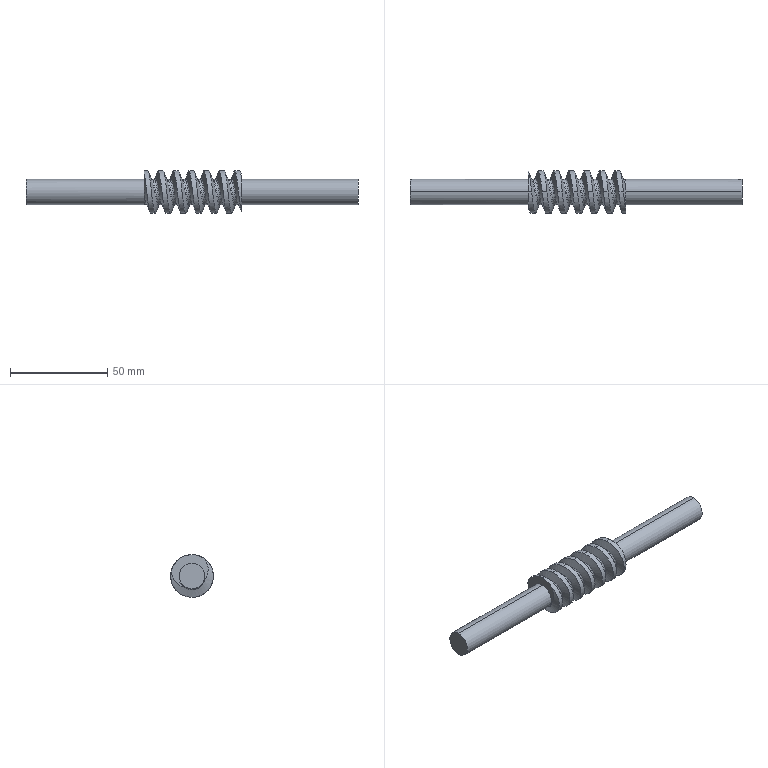Part | SolidWorks | features ICE 3, Helix 1, RefAxis 1, Revolution 1, SweepCut 1 | 1 solid | 27 faces | box 171 x 22 x 22 mm | volume 28864 mm3 | cylinder 18 | spline 5 | plane 4 | commonest cylinder face diameters 22 x14 13 x4